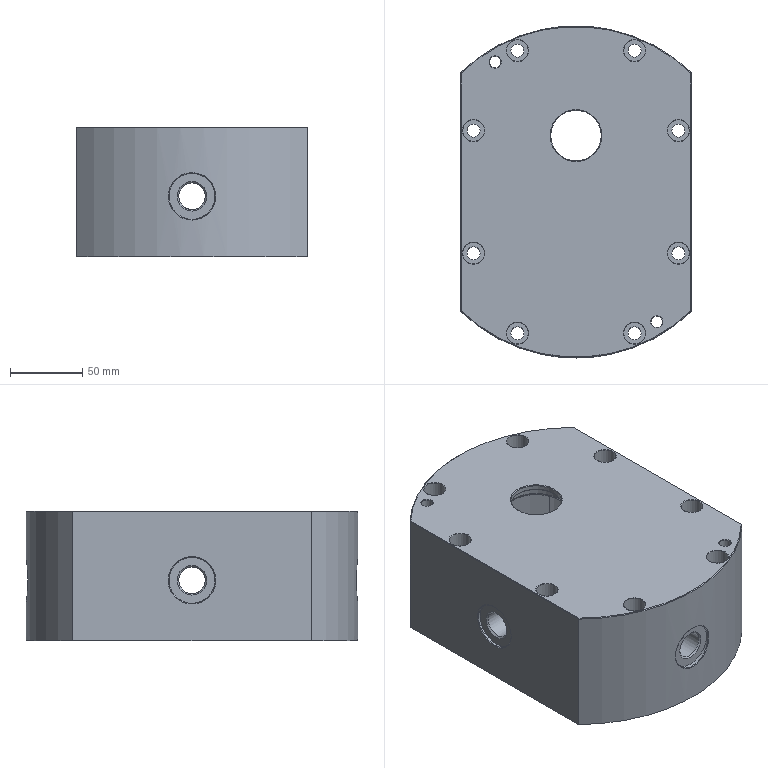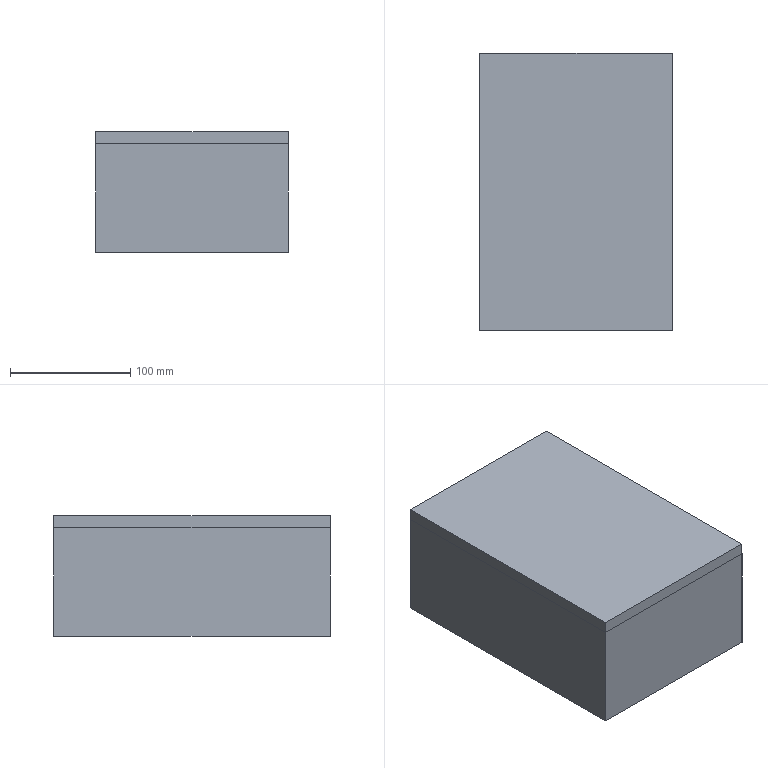CAM job | NX | 3+2 milling, drilling | part box 160 x 230 x 90 mm | stock box 160 x 230 x 100 mm
Tools:
number,name,description,diameter,corner_radius,flute_length,length,flutes
1,ZXZ,Milling Tool-5 Parameters,6.0,0.0,50.0,75.0,2
9,9.0ZT,Drilling Tool,9.0,0.0,35.0,50.0,2
8,7.8ZT,Drilling Tool,7.8,0.0,35.0,50.0,2
18,8.0JD,Milling Tool-5 Parameters,8.0,0.0,30.0,30.0,4
2,D50,Milling Tool-5 Parameters,50.0,0.0,50.0,75.0,2
10,D10,Milling Tool-5 Parameters,10.0,0.0,50.0,75.0,2
11,D10JING,Milling Tool-5 Parameters,10.0,0.0,50.0,75.0,2
7,D6A45,Milling Tool-5 Parameters,6.0,0.0,50.0,75.0,2
3,D3,Milling Tool-5 Parameters,3.0,0.0,50.0,75.0,2
5,D25R0.5,Milling Tool-5 Parameters,25.0,0.5,50.0,75.0,2
12,D12,Milling Tool-5 Parameters,12.0,0.0,50.0,75.0,2
Operations:
program,operation,operation_type,tool,method,geometry_group,spindle_rpm,surface_speed,feed_per_tooth,feed_cut,feed_plunge,cut_length_mm,path_length_mm,cut_time_min,machine_time_min
1,FLOOR_WALL,VolumeBased25DMillingOperation,D50,METHOD,A,1200.0,188.0,0.8333,2000.0,1000.0,84048.056,101883.151,42.324,44.108
1,FLOOR_WALL_COPY,VolumeBased25DMillingOperation,D50,METHOD,A,2500.0,392.0,0.2,1000.0,1000.0,1042.772,1166.772,1.043,1.055
1,HOLE_MILLING,CylinderMilling,D10,METHOD,A,3000.0,94.0,0.3667,2200.0,100.0,1761.999,1898.499,0.8009,0.8146
1,HOLE_MILLING_COPY,CylinderMilling,D10,METHOD,A,3000.0,94.0,0.3667,2200.0,100.0,2468.936,2622.436,1.122,1.138
1,HOLE_MILLING_COPY_1,CylinderMilling,D10JING,METHOD,A,5000.0,157.0,0.1,1000.0,100.0,95.013,229.013,0.095,0.1084
1,HOLE_MILLING_COPY_1_COPY,CylinderMilling,D10JING,METHOD,A,5000.0,157.0,0.1,1000.0,100.0,39.296,213.296,0.0393,0.0567
1,PLANAR_MILL,PlanarMilling,D6A45,METHOD,A,7500.0,141.0,0.0833,1250.0,100.0,457.474,1032.252,0.366,0.4235
1,PLANAR_MILL_COPY,PlanarMilling,D6A45,METHOD,A,7500.0,141.0,0.0833,1250.0,100.0,62.283,193.283,0.0498,0.0629
2,HOLE_MILLING_COPY_COPY,CylinderMilling,D10,METHOD,B,3000.0,94.0,0.3667,2200.0,100.0,14755.49,15935.568,6.707,6.825
2,HOLE_MILLING_COPY_COPY_COPY,CylinderMilling,D10,METHOD,B,3000.0,94.0,0.3667,2200.0,100.0,9087.411,9183.911,4.131,4.14
2,HOLE_MILLING_COPY_1_COPY_1,CylinderMilling,D10JING,METHOD,B,5000.0,157.0,0.1,1000.0,100.0,107.399,191.399,0.1074,0.1158
2,PLANAR_MILL_COPY_COPY,PlanarMilling,D6A45,METHOD,B,7500.0,141.0,0.0833,1250.0,100.0,513.924,1603.494,0.4111,0.5201
3,FLOOR_WALL_COPY_1,VolumeBased25DMillingOperation,D50,METHOD,C,1200.0,188.0,0.8333,2000.0,1000.0,48487.913,59439.44,24.331,25.426
3,FLOOR_WALL_COPY_COPY,VolumeBased25DMillingOperation,D50,METHOD,C,2500.0,392.0,0.2,1000.0,1000.0,1671.997,1725.997,1.672,1.677
3,DRILLING_COPY_1,Operation,ZXZ,METHOD,C,5000.0,94.0,0.025,250.0,0.0,40.0,676.066,0.16,0.2236
3,DRILLING_COPY,Operation,9.0ZT,METHOD,C,2000.0,56.0,0.0375,150.0,0.0,577.631,1736.917,3.851,3.967
3,DRILLING_COPY_COPY,Operation,7.8ZT,METHOD,C,2000.0,56.0,0.0375,150.0,0.0,52.687,380.395,0.3512,0.384
3,DRILLING_COPY_COPY_COPY,Operation,8.0JD,METHOD,C,800.0,20.0,0.0125,40.0,0.0,46.0,367.021,1.15,1.182
3,PLANAR_PROFILE,PlanarMilling,D3,METHOD,C,5000.0,47.0,0.11,1100.0,500.0,20558.032,20613.832,18.809,18.814
3,FLOOR_WALL_1,VolumeBased25DMillingOperation,D25R0.5,METHOD,C,2000.0,157.0,0.55,2200.0,1000.0,250780.736,265997.42,122.585,124.106
3,HOLE_MILLING_COPY_COPY_COPY_COPY,CylinderMilling,D12,METHOD,C,3000.0,113.0,0.25,1500.0,100.0,4110.519,4334.019,2.74,2.763
3,FLOOR_WALL_1_COPY,VolumeBased25DMillingOperation,D12,METHOD,C,4000.0,150.0,0.125,1000.0,500.0,4111.295,4330.569,4.174,4.196
3,FLOOR_WALL_1_COPY_COPY,VolumeBased25DMillingOperation,D12,METHOD,C,4000.0,150.0,0.125,1000.0,500.0,3669.138,3879.138,3.675,3.696
3,PLANAR_MILL_COPY_COPY_COPY,PlanarMilling,D6A45,METHOD,C,7500.0,141.0,0.0833,1250.0,100.0,2654.303,4115.73,2.123,2.27
3,CUTTER_COMP_12,CylinderMilling,D12,METHOD,C,4000.0,150.0,0.125,1000.0,100.0,114.121,346.122,0.1141,0.1373
4,HOLE_MILLING_COPY_2,CylinderMilling,D10,METHOD,D,3000.0,94.0,0.3667,2200.0,100.0,2461.748,2531.372,1.119,1.126
4,HOLE_MILLING_COPY_COPY_1,CylinderMilling,D10,METHOD,D,3000.0,94.0,0.3667,2200.0,100.0,2405.068,2490.029,1.093,1.102
4,HOLE_MILLING_COPY_1_COPY_2,CylinderMilling,D10JING,METHOD,D,5000.0,157.0,0.1,1000.0,100.0,95.013,161.013,0.095,0.1016
4,HOLE_MILLING_COPY_1_COPY_COPY,CylinderMilling,D10JING,METHOD,D,5000.0,157.0,0.1,1000.0,100.0,39.296,144.218,0.0393,0.0498
4,PLANAR_MILL_COPY_COPY_COPY_1,PlanarMilling,D6A45,METHOD,D,7500.0,141.0,0.0833,1250.0,100.0,65.383,128.383,0.0523,0.0586
4,PROFILE_3D,PlanarMilling,D6A45,METHOD,D,7500.0,141.0,0.0833,1250.0,100.0,103.734,160.516,0.083,0.0887